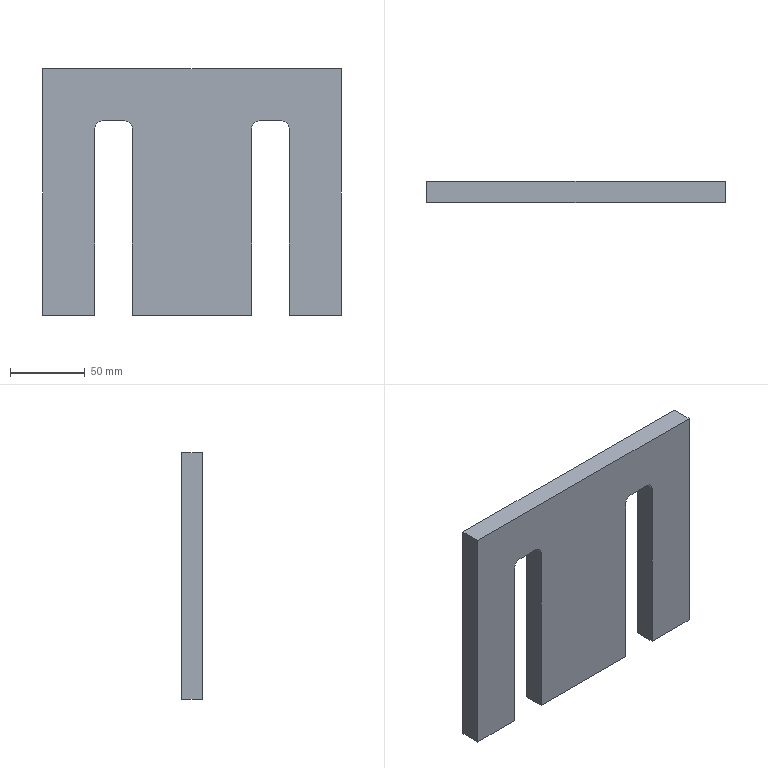Part | SolidWorks | features Extrusion 1, Fillet 1, ICE 1 | 1 solid | 18 faces | box 200 x 14 x 165 mm | volume 371300 mm3 | plane 14 | cylinder 4 | commonest cylinder face diameters 10 x4
STEP:
#1=CARTESIAN_POINT('',(40.,14.,-82.5));
#2=VERTEX_POINT('',#1);
#3=CARTESIAN_POINT('',(-40.,14.,-82.5));
#4=VERTEX_POINT('',#3);
#5=CARTESIAN_POINT('',(-100.,14.,-82.5));
#6=DIRECTION('',(-1.,0.,0.));
#7=VECTOR('',#6,1000.);
#8=LINE('',#5,#7);
#9=EDGE_CURVE('',#2,#4,#8,.T.);
#10=ORIENTED_EDGE('',*,*,#9,.F.);
#11=CARTESIAN_POINT('',(40.,0.,-82.5));
#12=VERTEX_POINT('',#11);
#13=CARTESIAN_POINT('',(40.,14.001,-82.5));
#14=DIRECTION('',(0.,-1.,0.));
#15=VECTOR('',#14,1000.);
#16=LINE('',#13,#15);
#17=EDGE_CURVE('',#2,#12,#16,.T.);
#18=ORIENTED_EDGE('',*,*,#17,.T.);
#19=CARTESIAN_POINT('',(-40.,0.,-82.5));
#20=VERTEX_POINT('',#19);
#21=CARTESIAN_POINT('',(-100.,0.,-82.5));
#22=DIRECTION('',(-1.,0.,0.));
#23=VECTOR('',#22,1000.);
#24=LINE('',#21,#23);
#25=EDGE_CURVE('',#12,#20,#24,.T.);
#26=ORIENTED_EDGE('',*,*,#25,.T.);
#27=CARTESIAN_POINT('',(-40.,14.001,-82.5));
#28=DIRECTION('',(0.,-1.,0.));
#29=VECTOR('',#28,1000.);
#30=LINE('',#27,#29);
#31=EDGE_CURVE('',#4,#20,#30,.T.);
#32=ORIENTED_EDGE('',*,*,#31,.F.);
#33=EDGE_LOOP('',(#10,#18,#26,#32));
#34=FACE_OUTER_BOUND('',#33,.T.);
#35=CARTESIAN_POINT('',(-100.,14.,-82.5));
#36=DIRECTION('',(0.,0.,1.));
#37=DIRECTION('',(1.,0.,0.));
#38=AXIS2_PLACEMENT_3D('',#35,#36,#37);
#39=PLANE('',#38);
#40=ADVANCED_FACE('',(#34),#39,.F.);
#41=CARTESIAN_POINT('',(100.,0.,-82.5));
#42=VERTEX_POINT('',#41);
#43=CARTESIAN_POINT('',(65.,0.,-82.5));
#44=VERTEX_POINT('',#43);
#45=CARTESIAN_POINT('',(-100.,0.,-82.5));
#46=DIRECTION('',(-1.,0.,0.));
#47=VECTOR('',#46,1000.);
#48=LINE('',#45,#47);
#49=EDGE_CURVE('',#42,#44,#48,.T.);
#50=ORIENTED_EDGE('',*,*,#49,.T.);
#51=CARTESIAN_POINT('',(65.,14.,-82.5));
#52=VERTEX_POINT('',#51);
#53=CARTESIAN_POINT('',(65.,14.001,-82.5));
#54=DIRECTION('',(0.,-1.,0.));
#55=VECTOR('',#54,1000.);
#56=LINE('',#53,#55);
#57=EDGE_CURVE('',#52,#44,#56,.T.);
#58=ORIENTED_EDGE('',*,*,#57,.F.);
#59=CARTESIAN_POINT('',(100.,14.,-82.5));
#60=VERTEX_POINT('',#59);
#61=CARTESIAN_POINT('',(-100.,14.,-82.5));
#62=DIRECTION('',(-1.,0.,0.));
#63=VECTOR('',#62,1000.);
#64=LINE('',#61,#63);
#65=EDGE_CURVE('',#60,#52,#64,.T.);
#66=ORIENTED_EDGE('',*,*,#65,.F.);
#67=CARTESIAN_POINT('',(100.,14.,-82.5));
#68=DIRECTION('',(0.,-1.,0.));
#69=VECTOR('',#68,1000.);
#70=LINE('',#67,#69);
#71=EDGE_CURVE('',#60,#42,#70,.T.);
#72=ORIENTED_EDGE('',*,*,#71,.T.);
#73=EDGE_LOOP('',(#50,#58,#66,#72));
#74=FACE_OUTER_BOUND('',#73,.T.);
#75=CARTESIAN_POINT('',(-100.,14.,-82.5));
#76=DIRECTION('',(0.,0.,1.));
#77=DIRECTION('',(1.,0.,0.));
#78=AXIS2_PLACEMENT_3D('',#75,#76,#77);
#79=PLANE('',#78);
#80=ADVANCED_FACE('',(#74),#79,.F.);
#81=CARTESIAN_POINT('',(100.,0.,82.5));
#82=VERTEX_POINT('',#81);
#83=CARTESIAN_POINT('',(100.,0.,82.5));
#84=DIRECTION('',(0.,0.,-1.));
#85=VECTOR('',#84,1000.);
#86=LINE('',#83,#85);
#87=EDGE_CURVE('',#82,#42,#86,.T.);
#88=ORIENTED_EDGE('',*,*,#87,.T.);
#89=ORIENTED_EDGE('',*,*,#71,.F.);
#90=CARTESIAN_POINT('',(100.,14.,82.5));
#91=VERTEX_POINT('',#90);
#92=CARTESIAN_POINT('',(100.,14.,82.5));
#93=DIRECTION('',(0.,0.,-1.));
#94=VECTOR('',#93,1000.);
#95=LINE('',#92,#94);
#96=EDGE_CURVE('',#91,#60,#95,.T.);
#97=ORIENTED_EDGE('',*,*,#96,.F.);
#98=CARTESIAN_POINT('',(100.,14.,82.5));
#99=DIRECTION('',(0.,-1.,0.));
#100=VECTOR('',#99,1000.);
#101=LINE('',#98,#100);
#102=EDGE_CURVE('',#91,#82,#101,.T.);
#103=ORIENTED_EDGE('',*,*,#102,.T.);
#104=EDGE_LOOP('',(#88,#89,#97,#103));
#105=FACE_OUTER_BOUND('',#104,.T.);
#106=CARTESIAN_POINT('',(100.,14.,82.5));
#107=DIRECTION('',(-1.,0.,0.));
#108=DIRECTION('',(0.,0.,1.));
#109=AXIS2_PLACEMENT_3D('',#106,#107,#108);
#110=PLANE('',#109);
#111=ADVANCED_FACE('',(#105),#110,.F.);
#112=CARTESIAN_POINT('',(-65.,14.,-82.5));
#113=VERTEX_POINT('',#112);
#114=CARTESIAN_POINT('',(-100.,14.,-82.5));
#115=VERTEX_POINT('',#114);
#116=CARTESIAN_POINT('',(-100.,14.,-82.5));
#117=DIRECTION('',(-1.,0.,0.));
#118=VECTOR('',#117,1000.);
#119=LINE('',#116,#118);
#120=EDGE_CURVE('',#113,#115,#119,.T.);
#121=ORIENTED_EDGE('',*,*,#120,.F.);
#122=CARTESIAN_POINT('',(-65.,0.,-82.5));
#123=VERTEX_POINT('',#122);
#124=CARTESIAN_POINT('',(-65.,14.001,-82.5));
#125=DIRECTION('',(0.,-1.,0.));
#126=VECTOR('',#125,1000.);
#127=LINE('',#124,#126);
#128=EDGE_CURVE('',#113,#123,#127,.T.);
#129=ORIENTED_EDGE('',*,*,#128,.T.);
#130=CARTESIAN_POINT('',(-100.,0.,-82.5));
#131=VERTEX_POINT('',#130);
#132=CARTESIAN_POINT('',(-100.,0.,-82.5));
#133=DIRECTION('',(-1.,0.,0.));
#134=VECTOR('',#133,1000.);
#135=LINE('',#132,#134);
#136=EDGE_CURVE('',#123,#131,#135,.T.);
#137=ORIENTED_EDGE('',*,*,#136,.T.);
#138=CARTESIAN_POINT('',(-100.,14.,-82.5));
#139=DIRECTION('',(0.,-1.,0.));
#140=VECTOR('',#139,1000.);
#141=LINE('',#138,#140);
#142=EDGE_CURVE('',#115,#131,#141,.T.);
#143=ORIENTED_EDGE('',*,*,#142,.F.);
#144=EDGE_LOOP('',(#121,#129,#137,#143));
#145=FACE_OUTER_BOUND('',#144,.T.);
#146=CARTESIAN_POINT('',(-100.,14.,-82.5));
#147=DIRECTION('',(0.,0.,1.));
#148=DIRECTION('',(1.,0.,0.));
#149=AXIS2_PLACEMENT_3D('',#146,#147,#148);
#150=PLANE('',#149);
#151=ADVANCED_FACE('',(#145),#150,.F.);
#152=CARTESIAN_POINT('',(-100.,0.,82.5));
#153=VERTEX_POINT('',#152);
#154=CARTESIAN_POINT('',(-100.,0.,82.5));
#155=DIRECTION('',(0.,0.,1.));
#156=VECTOR('',#155,1000.);
#157=LINE('',#154,#156);
#158=EDGE_CURVE('',#131,#153,#157,.T.);
#159=ORIENTED_EDGE('',*,*,#158,.T.);
#160=CARTESIAN_POINT('',(-100.,14.,82.5));
#161=VERTEX_POINT('',#160);
#162=CARTESIAN_POINT('',(-100.,14.,82.5));
#163=DIRECTION('',(0.,-1.,0.));
#164=VECTOR('',#163,1000.);
#165=LINE('',#162,#164);
#166=EDGE_CURVE('',#161,#153,#165,.T.);
#167=ORIENTED_EDGE('',*,*,#166,.F.);
#168=CARTESIAN_POINT('',(-100.,14.,82.5));
#169=DIRECTION('',(0.,0.,1.));
#170=VECTOR('',#169,1000.);
#171=LINE('',#168,#170);
#172=EDGE_CURVE('',#115,#161,#171,.T.);
#173=ORIENTED_EDGE('',*,*,#172,.F.);
#174=ORIENTED_EDGE('',*,*,#142,.T.);
#175=EDGE_LOOP('',(#159,#167,#173,#174));
#176=FACE_OUTER_BOUND('',#175,.T.);
#177=CARTESIAN_POINT('',(-100.,14.,82.5));
#178=DIRECTION('',(1.,0.,0.));
#179=DIRECTION('',(0.,0.,-1.));
#180=AXIS2_PLACEMENT_3D('',#177,#178,#179);
#181=PLANE('',#180);
#182=ADVANCED_FACE('',(#176),#181,.F.);
#183=CARTESIAN_POINT('',(-100.,0.,82.5));
#184=DIRECTION('',(1.,0.,0.));
#185=VECTOR('',#184,1000.);
#186=LINE('',#183,#185);
#187=EDGE_CURVE('',#153,#82,#186,.T.);
#188=ORIENTED_EDGE('',*,*,#187,.T.);
#189=ORIENTED_EDGE('',*,*,#102,.F.);
#190=CARTESIAN_POINT('',(-100.,14.,82.5));
#191=DIRECTION('',(1.,0.,0.));
#192=VECTOR('',#191,1000.);
#193=LINE('',#190,#192);
#194=EDGE_CURVE('',#161,#91,#193,.T.);
#195=ORIENTED_EDGE('',*,*,#194,.F.);
#196=ORIENTED_EDGE('',*,*,#166,.T.);
#197=EDGE_LOOP('',(#188,#189,#195,#196));
#198=FACE_OUTER_BOUND('',#197,.T.);
#199=CARTESIAN_POINT('',(-100.,14.,82.5));
#200=DIRECTION('',(0.,0.,-1.));
#201=DIRECTION('',(-1.,0.,0.));
#202=AXIS2_PLACEMENT_3D('',#199,#200,#201);
#203=PLANE('',#202);
#204=ADVANCED_FACE('',(#198),#203,.F.);
#205=CARTESIAN_POINT('',(45.,14.,47.5));
#206=VERTEX_POINT('',#205);
#207=CARTESIAN_POINT('',(60.,14.,47.5));
#208=VERTEX_POINT('',#207);
#209=CARTESIAN_POINT('',(65.,14.,47.5));
#210=DIRECTION('',(1.,0.,0.));
#211=VECTOR('',#210,1000.);
#212=LINE('',#209,#211);
#213=EDGE_CURVE('',#206,#208,#212,.T.);
#214=ORIENTED_EDGE('',*,*,#213,.F.);
#215=CARTESIAN_POINT('',(40.,14.,42.5));
#216=VERTEX_POINT('',#215);
#217=CARTESIAN_POINT('',(45.,14.,42.5));
#218=DIRECTION('',(0.,-1.,0.));
#219=DIRECTION('',(0.,0.,-1.));
#220=AXIS2_PLACEMENT_3D('',#217,#218,#219);
#221=CIRCLE('',#220,5.);
#222=EDGE_CURVE('',#206,#216,#221,.T.);
#223=ORIENTED_EDGE('',*,*,#222,.T.);
#224=CARTESIAN_POINT('',(40.,14.,47.5));
#225=DIRECTION('',(0.,0.,1.));
#226=VECTOR('',#225,1000.);
#227=LINE('',#224,#226);
#228=EDGE_CURVE('',#2,#216,#227,.T.);
#229=ORIENTED_EDGE('',*,*,#228,.F.);
#230=ORIENTED_EDGE('',*,*,#9,.T.);
#231=CARTESIAN_POINT('',(-40.,14.,42.5));
#232=VERTEX_POINT('',#231);
#233=CARTESIAN_POINT('',(-40.,14.,47.5));
#234=DIRECTION('',(0.,0.,-1.));
#235=VECTOR('',#234,1000.);
#236=LINE('',#233,#235);
#237=EDGE_CURVE('',#232,#4,#236,.T.);
#238=ORIENTED_EDGE('',*,*,#237,.F.);
#239=CARTESIAN_POINT('',(-45.,14.,47.5));
#240=VERTEX_POINT('',#239);
#241=CARTESIAN_POINT('',(-45.,14.,42.5));
#242=DIRECTION('',(0.,-1.,0.));
#243=DIRECTION('',(0.,0.,-1.));
#244=AXIS2_PLACEMENT_3D('',#241,#242,#243);
#245=CIRCLE('',#244,5.);
#246=EDGE_CURVE('',#232,#240,#245,.T.);
#247=ORIENTED_EDGE('',*,*,#246,.T.);
#248=CARTESIAN_POINT('',(-60.,14.,47.5));
#249=VERTEX_POINT('',#248);
#250=CARTESIAN_POINT('',(-65.,14.,47.5));
#251=DIRECTION('',(1.,0.,0.));
#252=VECTOR('',#251,1000.);
#253=LINE('',#250,#252);
#254=EDGE_CURVE('',#249,#240,#253,.T.);
#255=ORIENTED_EDGE('',*,*,#254,.F.);
#256=CARTESIAN_POINT('',(-65.,14.,42.5));
#257=VERTEX_POINT('',#256);
#258=CARTESIAN_POINT('',(-60.,14.,42.5));
#259=DIRECTION('',(0.,-1.,0.));
#260=DIRECTION('',(0.,0.,-1.));
#261=AXIS2_PLACEMENT_3D('',#258,#259,#260);
#262=CIRCLE('',#261,5.);
#263=EDGE_CURVE('',#249,#257,#262,.T.);
#264=ORIENTED_EDGE('',*,*,#263,.T.);
#265=CARTESIAN_POINT('',(-65.,14.,-82.5));
#266=DIRECTION('',(0.,0.,1.));
#267=VECTOR('',#266,1000.);
#268=LINE('',#265,#267);
#269=EDGE_CURVE('',#113,#257,#268,.T.);
#270=ORIENTED_EDGE('',*,*,#269,.F.);
#271=ORIENTED_EDGE('',*,*,#120,.T.);
#272=ORIENTED_EDGE('',*,*,#172,.T.);
#273=ORIENTED_EDGE('',*,*,#194,.T.);
#274=ORIENTED_EDGE('',*,*,#96,.T.);
#275=ORIENTED_EDGE('',*,*,#65,.T.);
#276=CARTESIAN_POINT('',(65.,14.,42.5));
#277=VERTEX_POINT('',#276);
#278=CARTESIAN_POINT('',(65.,14.,-82.5));
#279=DIRECTION('',(0.,0.,-1.));
#280=VECTOR('',#279,1000.);
#281=LINE('',#278,#280);
#282=EDGE_CURVE('',#277,#52,#281,.T.);
#283=ORIENTED_EDGE('',*,*,#282,.F.);
#284=CARTESIAN_POINT('',(60.,14.,42.5));
#285=DIRECTION('',(0.,-1.,0.));
#286=DIRECTION('',(0.,0.,-1.));
#287=AXIS2_PLACEMENT_3D('',#284,#285,#286);
#288=CIRCLE('',#287,5.);
#289=EDGE_CURVE('',#277,#208,#288,.T.);
#290=ORIENTED_EDGE('',*,*,#289,.T.);
#291=EDGE_LOOP('',(#214,#223,#229,#230,#238,#247,#255,#264,#270,#271,#272,#273,#274,#275,#283,#290));
#292=FACE_OUTER_BOUND('',#291,.T.);
#293=CARTESIAN_POINT('',(0.,14.,0.));
#294=DIRECTION('',(0.,-1.,0.));
#295=DIRECTION('',(0.,0.,-1.));
#296=AXIS2_PLACEMENT_3D('',#293,#294,#295);
#297=PLANE('',#296);
#298=ADVANCED_FACE('',(#292),#297,.F.);
#299=CARTESIAN_POINT('',(40.,0.,42.5));
#300=VERTEX_POINT('',#299);
#301=CARTESIAN_POINT('',(40.,0.,47.5));
#302=DIRECTION('',(0.,0.,-1.));
#303=VECTOR('',#302,1000.);
#304=LINE('',#301,#303);
#305=EDGE_CURVE('',#300,#12,#304,.T.);
#306=ORIENTED_EDGE('',*,*,#305,.F.);
#307=CARTESIAN_POINT('',(45.,0.,47.5));
#308=VERTEX_POINT('',#307);
#309=CARTESIAN_POINT('',(45.,0.,42.5));
#310=DIRECTION('',(0.,1.,0.));
#311=DIRECTION('',(0.,0.,-1.));
#312=AXIS2_PLACEMENT_3D('',#309,#310,#311);
#313=CIRCLE('',#312,5.);
#314=EDGE_CURVE('',#300,#308,#313,.T.);
#315=ORIENTED_EDGE('',*,*,#314,.T.);
#316=CARTESIAN_POINT('',(60.,0.,47.5));
#317=VERTEX_POINT('',#316);
#318=CARTESIAN_POINT('',(65.,0.,47.5));
#319=DIRECTION('',(-1.,0.,0.));
#320=VECTOR('',#319,1000.);
#321=LINE('',#318,#320);
#322=EDGE_CURVE('',#317,#308,#321,.T.);
#323=ORIENTED_EDGE('',*,*,#322,.F.);
#324=CARTESIAN_POINT('',(65.,0.,42.5));
#325=VERTEX_POINT('',#324);
#326=CARTESIAN_POINT('',(60.,0.,42.5));
#327=DIRECTION('',(0.,1.,0.));
#328=DIRECTION('',(0.,0.,-1.));
#329=AXIS2_PLACEMENT_3D('',#326,#327,#328);
#330=CIRCLE('',#329,5.);
#331=EDGE_CURVE('',#317,#325,#330,.T.);
#332=ORIENTED_EDGE('',*,*,#331,.T.);
#333=CARTESIAN_POINT('',(65.,0.,-82.5));
#334=DIRECTION('',(0.,0.,1.));
#335=VECTOR('',#334,1000.);
#336=LINE('',#333,#335);
#337=EDGE_CURVE('',#44,#325,#336,.T.);
#338=ORIENTED_EDGE('',*,*,#337,.F.);
#339=ORIENTED_EDGE('',*,*,#49,.F.);
#340=ORIENTED_EDGE('',*,*,#87,.F.);
#341=ORIENTED_EDGE('',*,*,#187,.F.);
#342=ORIENTED_EDGE('',*,*,#158,.F.);
#343=ORIENTED_EDGE('',*,*,#136,.F.);
#344=CARTESIAN_POINT('',(-65.,0.,42.5));
#345=VERTEX_POINT('',#344);
#346=CARTESIAN_POINT('',(-65.,0.,-82.5));
#347=DIRECTION('',(0.,0.,-1.));
#348=VECTOR('',#347,1000.);
#349=LINE('',#346,#348);
#350=EDGE_CURVE('',#345,#123,#349,.T.);
#351=ORIENTED_EDGE('',*,*,#350,.F.);
#352=CARTESIAN_POINT('',(-60.,0.,47.5));
#353=VERTEX_POINT('',#352);
#354=CARTESIAN_POINT('',(-60.,0.,42.5));
#355=DIRECTION('',(0.,1.,0.));
#356=DIRECTION('',(0.,0.,-1.));
#357=AXIS2_PLACEMENT_3D('',#354,#355,#356);
#358=CIRCLE('',#357,5.);
#359=EDGE_CURVE('',#345,#353,#358,.T.);
#360=ORIENTED_EDGE('',*,*,#359,.T.);
#361=CARTESIAN_POINT('',(-45.,0.,47.5));
#362=VERTEX_POINT('',#361);
#363=CARTESIAN_POINT('',(-65.,0.,47.5));
#364=DIRECTION('',(-1.,0.,0.));
#365=VECTOR('',#364,1000.);
#366=LINE('',#363,#365);
#367=EDGE_CURVE('',#362,#353,#366,.T.);
#368=ORIENTED_EDGE('',*,*,#367,.F.);
#369=CARTESIAN_POINT('',(-40.,0.,42.5));
#370=VERTEX_POINT('',#369);
#371=CARTESIAN_POINT('',(-45.,0.,42.5));
#372=DIRECTION('',(0.,1.,0.));
#373=DIRECTION('',(0.,0.,-1.));
#374=AXIS2_PLACEMENT_3D('',#371,#372,#373);
#375=CIRCLE('',#374,5.);
#376=EDGE_CURVE('',#362,#370,#375,.T.);
#377=ORIENTED_EDGE('',*,*,#376,.T.);
#378=CARTESIAN_POINT('',(-40.,0.,47.5));
#379=DIRECTION('',(0.,0.,1.));
#380=VECTOR('',#379,1000.);
#381=LINE('',#378,#380);
#382=EDGE_CURVE('',#20,#370,#381,.T.);
#383=ORIENTED_EDGE('',*,*,#382,.F.);
#384=ORIENTED_EDGE('',*,*,#25,.F.);
#385=EDGE_LOOP('',(#306,#315,#323,#332,#338,#339,#340,#341,#342,#343,#351,#360,#368,#377,#383,#384));
#386=FACE_OUTER_BOUND('',#385,.T.);
#387=CARTESIAN_POINT('',(0.,0.,0.));
#388=DIRECTION('',(0.,-1.,0.));
#389=DIRECTION('',(0.,0.,-1.));
#390=AXIS2_PLACEMENT_3D('',#387,#388,#389);
#391=PLANE('',#390);
#392=ADVANCED_FACE('',(#386),#391,.T.);
#393=ORIENTED_EDGE('',*,*,#382,.T.);
#394=CARTESIAN_POINT('',(-40.,14.,42.5));
#395=DIRECTION('',(0.,1.,0.));
#396=VECTOR('',#395,1000.);
#397=LINE('',#394,#396);
#398=EDGE_CURVE('',#370,#232,#397,.T.);
#399=ORIENTED_EDGE('',*,*,#398,.T.);
#400=ORIENTED_EDGE('',*,*,#237,.T.);
#401=ORIENTED_EDGE('',*,*,#31,.T.);
#402=EDGE_LOOP('',(#393,#399,#400,#401));
#403=FACE_OUTER_BOUND('',#402,.T.);
#404=CARTESIAN_POINT('',(-40.,14.001,47.5));
#405=DIRECTION('',(1.,0.,0.));
#406=DIRECTION('',(0.,0.,-1.));
#407=AXIS2_PLACEMENT_3D('',#404,#405,#406);
#408=PLANE('',#407);
#409=ADVANCED_FACE('',(#403),#408,.F.);
#410=ORIENTED_EDGE('',*,*,#269,.T.);
#411=CARTESIAN_POINT('',(-65.,0.,42.5));
#412=DIRECTION('',(0.,-1.,0.));
#413=VECTOR('',#412,1000.);
#414=LINE('',#411,#413);
#415=EDGE_CURVE('',#257,#345,#414,.T.);
#416=ORIENTED_EDGE('',*,*,#415,.T.);
#417=ORIENTED_EDGE('',*,*,#350,.T.);
#418=ORIENTED_EDGE('',*,*,#128,.F.);
#419=EDGE_LOOP('',(#410,#416,#417,#418));
#420=FACE_OUTER_BOUND('',#419,.T.);
#421=CARTESIAN_POINT('',(-65.,14.001,-82.5));
#422=DIRECTION('',(-1.,0.,0.));
#423=DIRECTION('',(0.,0.,1.));
#424=AXIS2_PLACEMENT_3D('',#421,#422,#423);
#425=PLANE('',#424);
#426=ADVANCED_FACE('',(#420),#425,.F.);
#427=ORIENTED_EDGE('',*,*,#254,.T.);
#428=CARTESIAN_POINT('',(-45.,0.,47.5));
#429=DIRECTION('',(0.,-1.,0.));
#430=VECTOR('',#429,1000.);
#431=LINE('',#428,#430);
#432=EDGE_CURVE('',#240,#362,#431,.T.);
#433=ORIENTED_EDGE('',*,*,#432,.T.);
#434=ORIENTED_EDGE('',*,*,#367,.T.);
#435=CARTESIAN_POINT('',(-60.,14.,47.5));
#436=DIRECTION('',(0.,1.,0.));
#437=VECTOR('',#436,1000.);
#438=LINE('',#435,#437);
#439=EDGE_CURVE('',#353,#249,#438,.T.);
#440=ORIENTED_EDGE('',*,*,#439,.T.);
#441=EDGE_LOOP('',(#427,#433,#434,#440));
#442=FACE_OUTER_BOUND('',#441,.T.);
#443=CARTESIAN_POINT('',(-65.,14.001,47.5));
#444=DIRECTION('',(0.,0.,1.));
#445=DIRECTION('',(1.,0.,0.));
#446=AXIS2_PLACEMENT_3D('',#443,#444,#445);
#447=PLANE('',#446);
#448=ADVANCED_FACE('',(#442),#447,.F.);
#449=ORIENTED_EDGE('',*,*,#228,.T.);
#450=CARTESIAN_POINT('',(40.,0.,42.5));
#451=DIRECTION('',(0.,-1.,0.));
#452=VECTOR('',#451,1000.);
#453=LINE('',#450,#452);
#454=EDGE_CURVE('',#216,#300,#453,.T.);
#455=ORIENTED_EDGE('',*,*,#454,.T.);
#456=ORIENTED_EDGE('',*,*,#305,.T.);
#457=ORIENTED_EDGE('',*,*,#17,.F.);
#458=EDGE_LOOP('',(#449,#455,#456,#457));
#459=FACE_OUTER_BOUND('',#458,.T.);
#460=CARTESIAN_POINT('',(40.,14.001,47.5));
#461=DIRECTION('',(-1.,0.,0.));
#462=DIRECTION('',(0.,0.,1.));
#463=AXIS2_PLACEMENT_3D('',#460,#461,#462);
#464=PLANE('',#463);
#465=ADVANCED_FACE('',(#459),#464,.F.);
#466=ORIENTED_EDGE('',*,*,#213,.T.);
#467=CARTESIAN_POINT('',(60.,0.,47.5));
#468=DIRECTION('',(0.,-1.,0.));
#469=VECTOR('',#468,1000.);
#470=LINE('',#467,#469);
#471=EDGE_CURVE('',#208,#317,#470,.T.);
#472=ORIENTED_EDGE('',*,*,#471,.T.);
#473=ORIENTED_EDGE('',*,*,#322,.T.);
#474=CARTESIAN_POINT('',(45.,14.,47.5));
#475=DIRECTION('',(0.,1.,0.));
#476=VECTOR('',#475,1000.);
#477=LINE('',#474,#476);
#478=EDGE_CURVE('',#308,#206,#477,.T.);
#479=ORIENTED_EDGE('',*,*,#478,.T.);
#480=EDGE_LOOP('',(#466,#472,#473,#479));
#481=FACE_OUTER_BOUND('',#480,.T.);
#482=CARTESIAN_POINT('',(65.,14.001,47.5));
#483=DIRECTION('',(0.,0.,1.));
#484=DIRECTION('',(1.,0.,0.));
#485=AXIS2_PLACEMENT_3D('',#482,#483,#484);
#486=PLANE('',#485);
#487=ADVANCED_FACE('',(#481),#486,.F.);
#488=ORIENTED_EDGE('',*,*,#337,.T.);
#489=CARTESIAN_POINT('',(65.,14.,42.5));
#490=DIRECTION('',(0.,1.,0.));
#491=VECTOR('',#490,1000.);
#492=LINE('',#489,#491);
#493=EDGE_CURVE('',#325,#277,#492,.T.);
#494=ORIENTED_EDGE('',*,*,#493,.T.);
#495=ORIENTED_EDGE('',*,*,#282,.T.);
#496=ORIENTED_EDGE('',*,*,#57,.T.);
#497=EDGE_LOOP('',(#488,#494,#495,#496));
#498=FACE_OUTER_BOUND('',#497,.T.);
#499=CARTESIAN_POINT('',(65.,14.001,-82.5));
#500=DIRECTION('',(1.,0.,0.));
#501=DIRECTION('',(0.,0.,-1.));
#502=AXIS2_PLACEMENT_3D('',#499,#500,#501);
#503=PLANE('',#502);
#504=ADVANCED_FACE('',(#498),#503,.F.);
#505=ORIENTED_EDGE('',*,*,#289,.F.);
#506=ORIENTED_EDGE('',*,*,#493,.F.);
#507=ORIENTED_EDGE('',*,*,#331,.F.);
#508=ORIENTED_EDGE('',*,*,#471,.F.);
#509=EDGE_LOOP('',(#505,#506,#507,#508));
#510=FACE_OUTER_BOUND('',#509,.T.);
#511=CARTESIAN_POINT('',(60.,14.001,42.5));
#512=DIRECTION('',(0.,1.,0.));
#513=DIRECTION('',(0.,0.,1.));
#514=AXIS2_PLACEMENT_3D('',#511,#512,#513);
#515=CYLINDRICAL_SURFACE('',#514,5.);
#516=ADVANCED_FACE('',(#510),#515,.F.);
#517=ORIENTED_EDGE('',*,*,#222,.F.);
#518=ORIENTED_EDGE('',*,*,#478,.F.);
#519=ORIENTED_EDGE('',*,*,#314,.F.);
#520=ORIENTED_EDGE('',*,*,#454,.F.);
#521=EDGE_LOOP('',(#517,#518,#519,#520));
#522=FACE_OUTER_BOUND('',#521,.T.);
#523=CARTESIAN_POINT('',(45.,14.001,42.5));
#524=DIRECTION('',(0.,1.,0.));
#525=DIRECTION('',(0.,0.,1.));
#526=AXIS2_PLACEMENT_3D('',#523,#524,#525);
#527=CYLINDRICAL_SURFACE('',#526,5.);
#528=ADVANCED_FACE('',(#522),#527,.F.);
#529=ORIENTED_EDGE('',*,*,#246,.F.);
#530=ORIENTED_EDGE('',*,*,#398,.F.);
#531=ORIENTED_EDGE('',*,*,#376,.F.);
#532=ORIENTED_EDGE('',*,*,#432,.F.);
#533=EDGE_LOOP('',(#529,#530,#531,#532));
#534=FACE_OUTER_BOUND('',#533,.T.);
#535=CARTESIAN_POINT('',(-45.,14.001,42.5));
#536=DIRECTION('',(0.,1.,0.));
#537=DIRECTION('',(0.,0.,1.));
#538=AXIS2_PLACEMENT_3D('',#535,#536,#537);
#539=CYLINDRICAL_SURFACE('',#538,5.);
#540=ADVANCED_FACE('',(#534),#539,.F.);
#541=ORIENTED_EDGE('',*,*,#263,.F.);
#542=ORIENTED_EDGE('',*,*,#439,.F.);
#543=ORIENTED_EDGE('',*,*,#359,.F.);
#544=ORIENTED_EDGE('',*,*,#415,.F.);
#545=EDGE_LOOP('',(#541,#542,#543,#544));
#546=FACE_OUTER_BOUND('',#545,.T.);
#547=CARTESIAN_POINT('',(-60.,14.001,42.5));
#548=DIRECTION('',(0.,1.,0.));
#549=DIRECTION('',(0.,0.,1.));
#550=AXIS2_PLACEMENT_3D('',#547,#548,#549);
#551=CYLINDRICAL_SURFACE('',#550,5.);
#552=ADVANCED_FACE('',(#546),#551,.F.);
#553=CLOSED_SHELL('',(#40,#80,#111,#151,#182,#204,#298,#392,#409,#426,#448,#465,#487,#504,#516,#528,#540,#552));
#554=MANIFOLD_SOLID_BREP('',#553);
#555=CARTESIAN_POINT('',(0.,0.,0.));
#556=DIRECTION('',(0.,0.,1.));
#557=DIRECTION('',(1.,0.,0.));
#558=AXIS2_PLACEMENT_3D('',#555,#556,#557);
#559=(LENGTH_UNIT()NAMED_UNIT(*)SI_UNIT(.MILLI.,.METRE.));
#560=UNCERTAINTY_MEASURE_WITH_UNIT(LENGTH_MEASURE(0.00001),#559,'','');
#561=(NAMED_UNIT(*)PLANE_ANGLE_UNIT()SI_UNIT($,.RADIAN.));
#562=(NAMED_UNIT(*)SI_UNIT($,.STERADIAN.)SOLID_ANGLE_UNIT());
#563=(GEOMETRIC_REPRESENTATION_CONTEXT(3)GLOBAL_UNCERTAINTY_ASSIGNED_CONTEXT((#560))GLOBAL_UNIT_ASSIGNED_CONTEXT((#559,#561,#562))REPRESENTATION_CONTEXT('',''));
#564=ADVANCED_BREP_SHAPE_REPRESENTATION('',(#554,#558),#563);